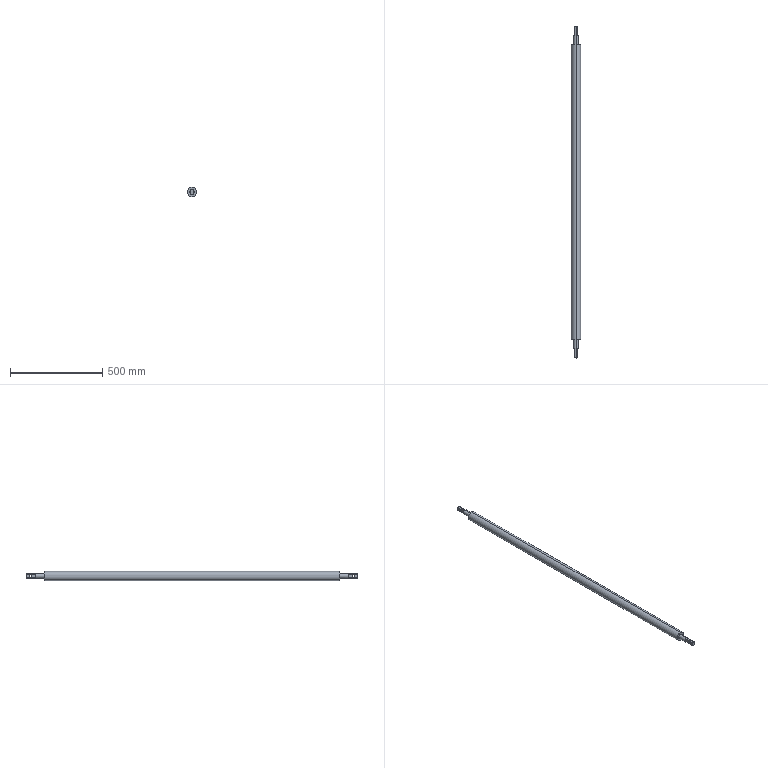Part | STEP file | Roller 11 | 1 solid | 22 faces | box 50 x 1800 x 50 mm | volume 3218952 mm3 | plane 12 | cylinder 10 | commonest cylinder face diameters 13 x4 25 x4 50 x2
STEP:
#1=CARTESIAN_POINT('',(6.703,-875.,6.5));
#2=VERTEX_POINT('',#1);
#3=CARTESIAN_POINT('',(6.703,-875.,-6.5));
#4=VERTEX_POINT('',#3);
#5=CARTESIAN_POINT('',(6.703,-875.,0.));
#6=DIRECTION('',(1.,0.,0.));
#7=DIRECTION('',(0.,0.,1.));
#8=AXIS2_PLACEMENT_3D('',#5,#6,#7);
#9=CIRCLE('',#8,6.5);
#10=EDGE_CURVE('',#2,#4,#9,.T.);
#11=ORIENTED_EDGE('',*,*,#10,.T.);
#12=CARTESIAN_POINT('',(-6.703,-875.,-6.5));
#13=VERTEX_POINT('',#12);
#14=CARTESIAN_POINT('',(29.297,-875.,-6.5));
#15=DIRECTION('',(-1.,0.,0.));
#16=VECTOR('',#15,1000.);
#17=LINE('',#14,#16);
#18=EDGE_CURVE('',#4,#13,#17,.T.);
#19=ORIENTED_EDGE('',*,*,#18,.T.);
#20=CARTESIAN_POINT('',(-6.703,-875.,6.5));
#21=VERTEX_POINT('',#20);
#22=CARTESIAN_POINT('',(-6.703,-875.,0.));
#23=DIRECTION('',(1.,0.,0.));
#24=DIRECTION('',(0.,0.,1.));
#25=AXIS2_PLACEMENT_3D('',#22,#23,#24);
#26=CIRCLE('',#25,6.5);
#27=EDGE_CURVE('',#21,#13,#26,.T.);
#28=ORIENTED_EDGE('',*,*,#27,.F.);
#29=CARTESIAN_POINT('',(29.297,-875.,6.5));
#30=DIRECTION('',(-1.,0.,0.));
#31=VECTOR('',#30,1000.);
#32=LINE('',#29,#31);
#33=EDGE_CURVE('',#2,#21,#32,.T.);
#34=ORIENTED_EDGE('',*,*,#33,.F.);
#35=EDGE_LOOP('',(#11,#19,#28,#34));
#36=FACE_OUTER_BOUND('',#35,.T.);
#37=CARTESIAN_POINT('',(29.297,-875.,0.));
#38=DIRECTION('',(-1.,0.,0.));
#39=DIRECTION('',(0.,0.,1.));
#40=AXIS2_PLACEMENT_3D('',#37,#38,#39);
#41=CYLINDRICAL_SURFACE('',#40,6.5);
#42=ADVANCED_FACE('',(#36),#41,.F.);
#43=CARTESIAN_POINT('',(6.703,875.,6.5));
#44=VERTEX_POINT('',#43);
#45=CARTESIAN_POINT('',(6.703,875.,-6.5));
#46=VERTEX_POINT('',#45);
#47=CARTESIAN_POINT('',(6.703,875.,0.));
#48=DIRECTION('',(1.,0.,0.));
#49=DIRECTION('',(0.,0.,-1.));
#50=AXIS2_PLACEMENT_3D('',#47,#48,#49);
#51=CIRCLE('',#50,6.5);
#52=EDGE_CURVE('',#44,#46,#51,.T.);
#53=ORIENTED_EDGE('',*,*,#52,.T.);
#54=CARTESIAN_POINT('',(-6.703,875.,-6.5));
#55=VERTEX_POINT('',#54);
#56=CARTESIAN_POINT('',(29.297,875.,-6.5));
#57=DIRECTION('',(-1.,0.,0.));
#58=VECTOR('',#57,1000.);
#59=LINE('',#56,#58);
#60=EDGE_CURVE('',#46,#55,#59,.T.);
#61=ORIENTED_EDGE('',*,*,#60,.T.);
#62=CARTESIAN_POINT('',(-6.703,875.,6.5));
#63=VERTEX_POINT('',#62);
#64=CARTESIAN_POINT('',(-6.703,875.,0.));
#65=DIRECTION('',(-1.,0.,0.));
#66=DIRECTION('',(0.,0.,1.));
#67=AXIS2_PLACEMENT_3D('',#64,#65,#66);
#68=CIRCLE('',#67,6.5);
#69=EDGE_CURVE('',#55,#63,#68,.T.);
#70=ORIENTED_EDGE('',*,*,#69,.T.);
#71=CARTESIAN_POINT('',(29.297,875.,6.5));
#72=DIRECTION('',(-1.,0.,0.));
#73=VECTOR('',#72,1000.);
#74=LINE('',#71,#73);
#75=EDGE_CURVE('',#44,#63,#74,.T.);
#76=ORIENTED_EDGE('',*,*,#75,.F.);
#77=EDGE_LOOP('',(#53,#61,#70,#76));
#78=FACE_OUTER_BOUND('',#77,.T.);
#79=CARTESIAN_POINT('',(29.297,875.,0.));
#80=DIRECTION('',(-1.,0.,0.));
#81=DIRECTION('',(0.,0.,1.));
#82=AXIS2_PLACEMENT_3D('',#79,#80,#81);
#83=CYLINDRICAL_SURFACE('',#82,6.5);
#84=ADVANCED_FACE('',(#78),#83,.F.);
#85=CARTESIAN_POINT('',(0.,-800.,-12.5));
#86=VERTEX_POINT('',#85);
#87=CARTESIAN_POINT('',(0.,-800.,12.5));
#88=VERTEX_POINT('',#87);
#89=CARTESIAN_POINT('',(0.,-800.,0.));
#90=DIRECTION('',(0.,-1.,0.));
#91=DIRECTION('',(0.,0.,1.));
#92=AXIS2_PLACEMENT_3D('',#89,#90,#91);
#93=CIRCLE('',#92,12.5);
#94=EDGE_CURVE('',#86,#88,#93,.T.);
#95=ORIENTED_EDGE('',*,*,#94,.T.);
#96=CARTESIAN_POINT('',(0.,-900.,12.5));
#97=VERTEX_POINT('',#96);
#98=CARTESIAN_POINT('',(0.,900.,12.5));
#99=DIRECTION('',(0.,-1.,0.));
#100=VECTOR('',#99,1000.);
#101=LINE('',#98,#100);
#102=EDGE_CURVE('',#88,#97,#101,.T.);
#103=ORIENTED_EDGE('',*,*,#102,.T.);
#104=CARTESIAN_POINT('',(6.703,-900.,10.551));
#105=VERTEX_POINT('',#104);
#106=CARTESIAN_POINT('',(0.,-900.,0.));
#107=DIRECTION('',(0.,1.,0.));
#108=DIRECTION('',(0.,0.,1.));
#109=AXIS2_PLACEMENT_3D('',#106,#107,#108);
#110=CIRCLE('',#109,12.5);
#111=EDGE_CURVE('',#97,#105,#110,.T.);
#112=ORIENTED_EDGE('',*,*,#111,.T.);
#113=CARTESIAN_POINT('',(6.703,-850.,10.551));
#114=VERTEX_POINT('',#113);
#115=CARTESIAN_POINT('',(6.703,900.,10.551));
#116=DIRECTION('',(0.,1.,0.));
#117=VECTOR('',#116,1000.);
#118=LINE('',#115,#117);
#119=EDGE_CURVE('',#105,#114,#118,.T.);
#120=ORIENTED_EDGE('',*,*,#119,.T.);
#121=CARTESIAN_POINT('',(6.703,-850.,-10.551));
#122=VERTEX_POINT('',#121);
#123=CARTESIAN_POINT('',(0.,-850.,0.));
#124=DIRECTION('',(0.,-1.,0.));
#125=DIRECTION('',(0.,0.,-1.));
#126=AXIS2_PLACEMENT_3D('',#123,#124,#125);
#127=CIRCLE('',#126,12.5);
#128=EDGE_CURVE('',#122,#114,#127,.T.);
#129=ORIENTED_EDGE('',*,*,#128,.F.);
#130=CARTESIAN_POINT('',(6.703,-900.,-10.551));
#131=VERTEX_POINT('',#130);
#132=CARTESIAN_POINT('',(6.703,900.,-10.551));
#133=DIRECTION('',(0.,-1.,0.));
#134=VECTOR('',#133,1000.);
#135=LINE('',#132,#134);
#136=EDGE_CURVE('',#122,#131,#135,.T.);
#137=ORIENTED_EDGE('',*,*,#136,.T.);
#138=CARTESIAN_POINT('',(0.,-900.,-12.5));
#139=VERTEX_POINT('',#138);
#140=CARTESIAN_POINT('',(0.,-900.,0.));
#141=DIRECTION('',(0.,1.,0.));
#142=DIRECTION('',(0.,0.,1.));
#143=AXIS2_PLACEMENT_3D('',#140,#141,#142);
#144=CIRCLE('',#143,12.5);
#145=EDGE_CURVE('',#131,#139,#144,.T.);
#146=ORIENTED_EDGE('',*,*,#145,.T.);
#147=CARTESIAN_POINT('',(0.,900.,-12.5));
#148=DIRECTION('',(0.,-1.,0.));
#149=VECTOR('',#148,1000.);
#150=LINE('',#147,#149);
#151=EDGE_CURVE('',#86,#139,#150,.T.);
#152=ORIENTED_EDGE('',*,*,#151,.F.);
#153=EDGE_LOOP('',(#95,#103,#112,#120,#129,#137,#146,#152));
#154=FACE_OUTER_BOUND('',#153,.T.);
#155=CARTESIAN_POINT('',(0.,900.,0.));
#156=DIRECTION('',(0.,-1.,0.));
#157=DIRECTION('',(0.,0.,-1.));
#158=AXIS2_PLACEMENT_3D('',#155,#156,#157);
#159=CYLINDRICAL_SURFACE('',#158,12.5);
#160=ADVANCED_FACE('',(#154),#159,.T.);
#161=CARTESIAN_POINT('',(0.,800.,25.));
#162=VERTEX_POINT('',#161);
#163=CARTESIAN_POINT('',(0.,800.,-25.));
#164=VERTEX_POINT('',#163);
#165=CARTESIAN_POINT('',(0.,800.,0.));
#166=DIRECTION('',(0.,1.,0.));
#167=DIRECTION('',(0.,0.,1.));
#168=AXIS2_PLACEMENT_3D('',#165,#166,#167);
#169=CIRCLE('',#168,25.);
#170=EDGE_CURVE('',#162,#164,#169,.T.);
#171=ORIENTED_EDGE('',*,*,#170,.F.);
#172=CARTESIAN_POINT('',(0.,-800.,25.));
#173=VERTEX_POINT('',#172);
#174=CARTESIAN_POINT('',(0.,800.,25.));
#175=DIRECTION('',(0.,-1.,0.));
#176=VECTOR('',#175,1000.);
#177=LINE('',#174,#176);
#178=EDGE_CURVE('',#162,#173,#177,.T.);
#179=ORIENTED_EDGE('',*,*,#178,.T.);
#180=CARTESIAN_POINT('',(0.,-800.,-25.));
#181=VERTEX_POINT('',#180);
#182=CARTESIAN_POINT('',(0.,-800.,0.));
#183=DIRECTION('',(0.,1.,0.));
#184=DIRECTION('',(0.,0.,1.));
#185=AXIS2_PLACEMENT_3D('',#182,#183,#184);
#186=CIRCLE('',#185,25.);
#187=EDGE_CURVE('',#173,#181,#186,.T.);
#188=ORIENTED_EDGE('',*,*,#187,.T.);
#189=CARTESIAN_POINT('',(0.,800.,-25.));
#190=DIRECTION('',(0.,-1.,0.));
#191=VECTOR('',#190,1000.);
#192=LINE('',#189,#191);
#193=EDGE_CURVE('',#164,#181,#192,.T.);
#194=ORIENTED_EDGE('',*,*,#193,.F.);
#195=EDGE_LOOP('',(#171,#179,#188,#194));
#196=FACE_OUTER_BOUND('',#195,.T.);
#197=CARTESIAN_POINT('',(0.,800.,0.));
#198=DIRECTION('',(0.,-1.,0.));
#199=DIRECTION('',(0.,0.,-1.));
#200=AXIS2_PLACEMENT_3D('',#197,#198,#199);
#201=CYLINDRICAL_SURFACE('',#200,25.);
#202=ADVANCED_FACE('',(#196),#201,.T.);
#203=CARTESIAN_POINT('',(0.,900.,12.5));
#204=VERTEX_POINT('',#203);
#205=CARTESIAN_POINT('',(6.703,900.,10.551));
#206=VERTEX_POINT('',#205);
#207=CARTESIAN_POINT('',(0.,900.,0.));
#208=DIRECTION('',(0.,1.,0.));
#209=DIRECTION('',(0.,0.,1.));
#210=AXIS2_PLACEMENT_3D('',#207,#208,#209);
#211=CIRCLE('',#210,12.5);
#212=EDGE_CURVE('',#204,#206,#211,.T.);
#213=ORIENTED_EDGE('',*,*,#212,.F.);
#214=CARTESIAN_POINT('',(0.,800.,12.5));
#215=VERTEX_POINT('',#214);
#216=CARTESIAN_POINT('',(0.,900.,12.5));
#217=DIRECTION('',(0.,-1.,0.));
#218=VECTOR('',#217,1000.);
#219=LINE('',#216,#218);
#220=EDGE_CURVE('',#204,#215,#219,.T.);
#221=ORIENTED_EDGE('',*,*,#220,.T.);
#222=CARTESIAN_POINT('',(0.,800.,-12.5));
#223=VERTEX_POINT('',#222);
#224=CARTESIAN_POINT('',(0.,800.,0.));
#225=DIRECTION('',(0.,-1.,0.));
#226=DIRECTION('',(0.,0.,1.));
#227=AXIS2_PLACEMENT_3D('',#224,#225,#226);
#228=CIRCLE('',#227,12.5);
#229=EDGE_CURVE('',#223,#215,#228,.T.);
#230=ORIENTED_EDGE('',*,*,#229,.F.);
#231=CARTESIAN_POINT('',(0.,900.,-12.5));
#232=VERTEX_POINT('',#231);
#233=CARTESIAN_POINT('',(0.,900.,-12.5));
#234=DIRECTION('',(0.,-1.,0.));
#235=VECTOR('',#234,1000.);
#236=LINE('',#233,#235);
#237=EDGE_CURVE('',#232,#223,#236,.T.);
#238=ORIENTED_EDGE('',*,*,#237,.F.);
#239=CARTESIAN_POINT('',(6.703,900.,-10.551));
#240=VERTEX_POINT('',#239);
#241=CARTESIAN_POINT('',(0.,900.,0.));
#242=DIRECTION('',(0.,1.,0.));
#243=DIRECTION('',(0.,0.,1.));
#244=AXIS2_PLACEMENT_3D('',#241,#242,#243);
#245=CIRCLE('',#244,12.5);
#246=EDGE_CURVE('',#240,#232,#245,.T.);
#247=ORIENTED_EDGE('',*,*,#246,.F.);
#248=CARTESIAN_POINT('',(6.703,850.,-10.551));
#249=VERTEX_POINT('',#248);
#250=CARTESIAN_POINT('',(6.703,900.,-10.551));
#251=DIRECTION('',(0.,1.,0.));
#252=VECTOR('',#251,1000.);
#253=LINE('',#250,#252);
#254=EDGE_CURVE('',#249,#240,#253,.T.);
#255=ORIENTED_EDGE('',*,*,#254,.F.);
#256=CARTESIAN_POINT('',(6.703,850.,10.551));
#257=VERTEX_POINT('',#256);
#258=CARTESIAN_POINT('',(0.,850.,0.));
#259=DIRECTION('',(0.,1.,0.));
#260=DIRECTION('',(0.,0.,1.));
#261=AXIS2_PLACEMENT_3D('',#258,#259,#260);
#262=CIRCLE('',#261,12.5);
#263=EDGE_CURVE('',#257,#249,#262,.T.);
#264=ORIENTED_EDGE('',*,*,#263,.F.);
#265=CARTESIAN_POINT('',(6.703,900.,10.551));
#266=DIRECTION('',(0.,-1.,0.));
#267=VECTOR('',#266,1000.);
#268=LINE('',#265,#267);
#269=EDGE_CURVE('',#206,#257,#268,.T.);
#270=ORIENTED_EDGE('',*,*,#269,.F.);
#271=EDGE_LOOP('',(#213,#221,#230,#238,#247,#255,#264,#270));
#272=FACE_OUTER_BOUND('',#271,.T.);
#273=CARTESIAN_POINT('',(0.,900.,0.));
#274=DIRECTION('',(0.,-1.,0.));
#275=DIRECTION('',(0.,0.,-1.));
#276=AXIS2_PLACEMENT_3D('',#273,#274,#275);
#277=CYLINDRICAL_SURFACE('',#276,12.5);
#278=ADVANCED_FACE('',(#272),#277,.T.);
#279=ORIENTED_EDGE('',*,*,#220,.F.);
#280=CARTESIAN_POINT('',(-6.703,900.,10.551));
#281=VERTEX_POINT('',#280);
#282=CARTESIAN_POINT('',(0.,900.,0.));
#283=DIRECTION('',(0.,1.,0.));
#284=DIRECTION('',(0.,0.,1.));
#285=AXIS2_PLACEMENT_3D('',#282,#283,#284);
#286=CIRCLE('',#285,12.5);
#287=EDGE_CURVE('',#281,#204,#286,.T.);
#288=ORIENTED_EDGE('',*,*,#287,.F.);
#289=CARTESIAN_POINT('',(-6.703,850.,10.551));
#290=VERTEX_POINT('',#289);
#291=CARTESIAN_POINT('',(-6.703,900.,10.551));
#292=DIRECTION('',(0.,1.,0.));
#293=VECTOR('',#292,1000.);
#294=LINE('',#291,#293);
#295=EDGE_CURVE('',#290,#281,#294,.T.);
#296=ORIENTED_EDGE('',*,*,#295,.F.);
#297=CARTESIAN_POINT('',(-6.703,850.,-10.551));
#298=VERTEX_POINT('',#297);
#299=CARTESIAN_POINT('',(0.,850.,0.));
#300=DIRECTION('',(0.,1.,0.));
#301=DIRECTION('',(0.,0.,1.));
#302=AXIS2_PLACEMENT_3D('',#299,#300,#301);
#303=CIRCLE('',#302,12.5);
#304=EDGE_CURVE('',#298,#290,#303,.T.);
#305=ORIENTED_EDGE('',*,*,#304,.F.);
#306=CARTESIAN_POINT('',(-6.703,900.,-10.551));
#307=VERTEX_POINT('',#306);
#308=CARTESIAN_POINT('',(-6.703,900.,-10.551));
#309=DIRECTION('',(0.,-1.,0.));
#310=VECTOR('',#309,1000.);
#311=LINE('',#308,#310);
#312=EDGE_CURVE('',#307,#298,#311,.T.);
#313=ORIENTED_EDGE('',*,*,#312,.F.);
#314=CARTESIAN_POINT('',(0.,900.,0.));
#315=DIRECTION('',(0.,1.,0.));
#316=DIRECTION('',(0.,0.,1.));
#317=AXIS2_PLACEMENT_3D('',#314,#315,#316);
#318=CIRCLE('',#317,12.5);
#319=EDGE_CURVE('',#232,#307,#318,.T.);
#320=ORIENTED_EDGE('',*,*,#319,.F.);
#321=ORIENTED_EDGE('',*,*,#237,.T.);
#322=CARTESIAN_POINT('',(0.,800.,0.));
#323=DIRECTION('',(0.,-1.,0.));
#324=DIRECTION('',(0.,0.,1.));
#325=AXIS2_PLACEMENT_3D('',#322,#323,#324);
#326=CIRCLE('',#325,12.5);
#327=EDGE_CURVE('',#215,#223,#326,.T.);
#328=ORIENTED_EDGE('',*,*,#327,.F.);
#329=EDGE_LOOP('',(#279,#288,#296,#305,#313,#320,#321,#328));
#330=FACE_OUTER_BOUND('',#329,.T.);
#331=CARTESIAN_POINT('',(0.,900.,0.));
#332=DIRECTION('',(0.,-1.,0.));
#333=DIRECTION('',(0.,0.,-1.));
#334=AXIS2_PLACEMENT_3D('',#331,#332,#333);
#335=CYLINDRICAL_SURFACE('',#334,12.5);
#336=ADVANCED_FACE('',(#330),#335,.T.);
#337=ORIENTED_EDGE('',*,*,#246,.T.);
#338=ORIENTED_EDGE('',*,*,#319,.T.);
#339=CARTESIAN_POINT('',(-6.703,900.,0.));
#340=DIRECTION('',(0.,0.,1.));
#341=VECTOR('',#340,1000.);
#342=LINE('',#339,#341);
#343=EDGE_CURVE('',#307,#281,#342,.T.);
#344=ORIENTED_EDGE('',*,*,#343,.T.);
#345=ORIENTED_EDGE('',*,*,#287,.T.);
#346=ORIENTED_EDGE('',*,*,#212,.T.);
#347=CARTESIAN_POINT('',(6.703,900.,0.));
#348=DIRECTION('',(0.,0.,-1.));
#349=VECTOR('',#348,1000.);
#350=LINE('',#347,#349);
#351=EDGE_CURVE('',#206,#240,#350,.T.);
#352=ORIENTED_EDGE('',*,*,#351,.T.);
#353=EDGE_LOOP('',(#337,#338,#344,#345,#346,#352));
#354=FACE_OUTER_BOUND('',#353,.T.);
#355=CARTESIAN_POINT('',(0.,900.,0.));
#356=DIRECTION('',(0.,1.,0.));
#357=DIRECTION('',(0.,0.,1.));
#358=AXIS2_PLACEMENT_3D('',#355,#356,#357);
#359=PLANE('',#358);
#360=ADVANCED_FACE('',(#354),#359,.T.);
#361=ORIENTED_EDGE('',*,*,#178,.F.);
#362=CARTESIAN_POINT('',(0.,800.,0.));
#363=DIRECTION('',(0.,1.,0.));
#364=DIRECTION('',(0.,0.,1.));
#365=AXIS2_PLACEMENT_3D('',#362,#363,#364);
#366=CIRCLE('',#365,25.);
#367=EDGE_CURVE('',#164,#162,#366,.T.);
#368=ORIENTED_EDGE('',*,*,#367,.F.);
#369=ORIENTED_EDGE('',*,*,#193,.T.);
#370=CARTESIAN_POINT('',(0.,-800.,0.));
#371=DIRECTION('',(0.,1.,0.));
#372=DIRECTION('',(0.,0.,1.));
#373=AXIS2_PLACEMENT_3D('',#370,#371,#372);
#374=CIRCLE('',#373,25.);
#375=EDGE_CURVE('',#181,#173,#374,.T.);
#376=ORIENTED_EDGE('',*,*,#375,.T.);
#377=EDGE_LOOP('',(#361,#368,#369,#376));
#378=FACE_OUTER_BOUND('',#377,.T.);
#379=CARTESIAN_POINT('',(0.,800.,0.));
#380=DIRECTION('',(0.,-1.,0.));
#381=DIRECTION('',(0.,0.,-1.));
#382=AXIS2_PLACEMENT_3D('',#379,#380,#381);
#383=CYLINDRICAL_SURFACE('',#382,25.);
#384=ADVANCED_FACE('',(#378),#383,.T.);
#385=ORIENTED_EDGE('',*,*,#229,.T.);
#386=ORIENTED_EDGE('',*,*,#327,.T.);
#387=EDGE_LOOP('',(#385,#386));
#388=FACE_BOUND('',#387,.T.);
#389=ORIENTED_EDGE('',*,*,#367,.T.);
#390=ORIENTED_EDGE('',*,*,#170,.T.);
#391=EDGE_LOOP('',(#389,#390));
#392=FACE_OUTER_BOUND('',#391,.T.);
#393=CARTESIAN_POINT('',(0.,800.,0.));
#394=DIRECTION('',(0.,1.,0.));
#395=DIRECTION('',(0.,0.,1.));
#396=AXIS2_PLACEMENT_3D('',#393,#394,#395);
#397=PLANE('',#396);
#398=ADVANCED_FACE('',(#388,#392),#397,.T.);
#399=ORIENTED_EDGE('',*,*,#94,.F.);
#400=CARTESIAN_POINT('',(0.,-800.,0.));
#401=DIRECTION('',(0.,-1.,0.));
#402=DIRECTION('',(0.,0.,1.));
#403=AXIS2_PLACEMENT_3D('',#400,#401,#402);
#404=CIRCLE('',#403,12.5);
#405=EDGE_CURVE('',#88,#86,#404,.T.);
#406=ORIENTED_EDGE('',*,*,#405,.F.);
#407=EDGE_LOOP('',(#399,#406));
#408=FACE_BOUND('',#407,.T.);
#409=ORIENTED_EDGE('',*,*,#375,.F.);
#410=ORIENTED_EDGE('',*,*,#187,.F.);
#411=EDGE_LOOP('',(#409,#410));
#412=FACE_OUTER_BOUND('',#411,.T.);
#413=CARTESIAN_POINT('',(0.,-800.,0.));
#414=DIRECTION('',(0.,1.,0.));
#415=DIRECTION('',(0.,0.,1.));
#416=AXIS2_PLACEMENT_3D('',#413,#414,#415);
#417=PLANE('',#416);
#418=ADVANCED_FACE('',(#408,#412),#417,.F.);
#419=CARTESIAN_POINT('',(-6.703,-900.,10.551));
#420=VERTEX_POINT('',#419);
#421=CARTESIAN_POINT('',(0.,-900.,0.));
#422=DIRECTION('',(0.,1.,0.));
#423=DIRECTION('',(0.,0.,1.));
#424=AXIS2_PLACEMENT_3D('',#421,#422,#423);
#425=CIRCLE('',#424,12.5);
#426=EDGE_CURVE('',#420,#97,#425,.T.);
#427=ORIENTED_EDGE('',*,*,#426,.F.);
#428=CARTESIAN_POINT('',(-6.703,-900.,-10.551));
#429=VERTEX_POINT('',#428);
#430=CARTESIAN_POINT('',(-6.703,-900.,-19.04));
#431=DIRECTION('',(0.,0.,1.));
#432=VECTOR('',#431,1000.);
#433=LINE('',#430,#432);
#434=EDGE_CURVE('',#429,#420,#433,.T.);
#435=ORIENTED_EDGE('',*,*,#434,.F.);
#436=CARTESIAN_POINT('',(0.,-900.,0.));
#437=DIRECTION('',(0.,1.,0.));
#438=DIRECTION('',(0.,0.,1.));
#439=AXIS2_PLACEMENT_3D('',#436,#437,#438);
#440=CIRCLE('',#439,12.5);
#441=EDGE_CURVE('',#139,#429,#440,.T.);
#442=ORIENTED_EDGE('',*,*,#441,.F.);
#443=ORIENTED_EDGE('',*,*,#145,.F.);
#444=CARTESIAN_POINT('',(6.703,-900.,-19.04));
#445=DIRECTION('',(0.,0.,-1.));
#446=VECTOR('',#445,1000.);
#447=LINE('',#444,#446);
#448=EDGE_CURVE('',#105,#131,#447,.T.);
#449=ORIENTED_EDGE('',*,*,#448,.F.);
#450=ORIENTED_EDGE('',*,*,#111,.F.);
#451=EDGE_LOOP('',(#427,#435,#442,#443,#449,#450));
#452=FACE_OUTER_BOUND('',#451,.T.);
#453=CARTESIAN_POINT('',(0.,-900.,0.));
#454=DIRECTION('',(0.,1.,0.));
#455=DIRECTION('',(0.,0.,1.));
#456=AXIS2_PLACEMENT_3D('',#453,#454,#455);
#457=PLANE('',#456);
#458=ADVANCED_FACE('',(#452),#457,.F.);
#459=ORIENTED_EDGE('',*,*,#102,.F.);
#460=ORIENTED_EDGE('',*,*,#405,.T.);
#461=ORIENTED_EDGE('',*,*,#151,.T.);
#462=ORIENTED_EDGE('',*,*,#441,.T.);
#463=CARTESIAN_POINT('',(-6.703,-850.,-10.551));
#464=VERTEX_POINT('',#463);
#465=CARTESIAN_POINT('',(-6.703,900.,-10.551));
#466=DIRECTION('',(0.,1.,0.));
#467=VECTOR('',#466,1000.);
#468=LINE('',#465,#467);
#469=EDGE_CURVE('',#429,#464,#468,.T.);
#470=ORIENTED_EDGE('',*,*,#469,.T.);
#471=CARTESIAN_POINT('',(-6.703,-850.,10.551));
#472=VERTEX_POINT('',#471);
#473=CARTESIAN_POINT('',(0.,-850.,0.));
#474=DIRECTION('',(0.,-1.,0.));
#475=DIRECTION('',(0.,0.,-1.));
#476=AXIS2_PLACEMENT_3D('',#473,#474,#475);
#477=CIRCLE('',#476,12.5);
#478=EDGE_CURVE('',#472,#464,#477,.T.);
#479=ORIENTED_EDGE('',*,*,#478,.F.);
#480=CARTESIAN_POINT('',(-6.703,900.,10.551));
#481=DIRECTION('',(0.,-1.,0.));
#482=VECTOR('',#481,1000.);
#483=LINE('',#480,#482);
#484=EDGE_CURVE('',#472,#420,#483,.T.);
#485=ORIENTED_EDGE('',*,*,#484,.T.);
#486=ORIENTED_EDGE('',*,*,#426,.T.);
#487=EDGE_LOOP('',(#459,#460,#461,#462,#470,#479,#485,#486));
#488=FACE_OUTER_BOUND('',#487,.T.);
#489=CARTESIAN_POINT('',(0.,900.,0.));
#490=DIRECTION('',(0.,-1.,0.));
#491=DIRECTION('',(0.,0.,-1.));
#492=AXIS2_PLACEMENT_3D('',#489,#490,#491);
#493=CYLINDRICAL_SURFACE('',#492,12.5);
#494=ADVANCED_FACE('',(#488),#493,.T.);
#495=ORIENTED_EDGE('',*,*,#52,.F.);
#496=CARTESIAN_POINT('',(6.703,875.,0.));
#497=DIRECTION('',(1.,0.,0.));
#498=DIRECTION('',(0.,0.,-1.));
#499=AXIS2_PLACEMENT_3D('',#496,#497,#498);
#500=CIRCLE('',#499,6.5);
#501=EDGE_CURVE('',#46,#44,#500,.T.);
#502=ORIENTED_EDGE('',*,*,#501,.F.);
#503=EDGE_LOOP('',(#495,#502));
#504=FACE_BOUND('',#503,.T.);
#505=ORIENTED_EDGE('',*,*,#269,.T.);
#506=CARTESIAN_POINT('',(6.703,850.,-19.04));
#507=DIRECTION('',(0.,0.,-1.));
#508=VECTOR('',#507,1000.);
#509=LINE('',#506,#508);
#510=EDGE_CURVE('',#257,#249,#509,.T.);
#511=ORIENTED_EDGE('',*,*,#510,.T.);
#512=ORIENTED_EDGE('',*,*,#254,.T.);
#513=ORIENTED_EDGE('',*,*,#351,.F.);
#514=EDGE_LOOP('',(#505,#511,#512,#513));
#515=FACE_OUTER_BOUND('',#514,.T.);
#516=CARTESIAN_POINT('',(6.703,850.,-19.04));
#517=DIRECTION('',(1.,0.,0.));
#518=DIRECTION('',(0.,0.,-1.));
#519=AXIS2_PLACEMENT_3D('',#516,#517,#518);
#520=PLANE('',#519);
#521=ADVANCED_FACE('',(#504,#515),#520,.T.);
#522=ORIENTED_EDGE('',*,*,#263,.T.);
#523=ORIENTED_EDGE('',*,*,#510,.F.);
#524=EDGE_LOOP('',(#522,#523));
#525=FACE_OUTER_BOUND('',#524,.T.);
#526=CARTESIAN_POINT('',(0.,850.,0.));
#527=DIRECTION('',(0.,1.,0.));
#528=DIRECTION('',(0.,0.,1.));
#529=AXIS2_PLACEMENT_3D('',#526,#527,#528);
#530=PLANE('',#529);
#531=ADVANCED_FACE('',(#525),#530,.T.);
#532=ORIENTED_EDGE('',*,*,#304,.T.);
#533=CARTESIAN_POINT('',(-6.703,850.,-19.04));
#534=DIRECTION('',(0.,0.,1.));
#535=VECTOR('',#534,1000.);
#536=LINE('',#533,#535);
#537=EDGE_CURVE('',#298,#290,#536,.T.);
#538=ORIENTED_EDGE('',*,*,#537,.F.);
#539=EDGE_LOOP('',(#532,#538));
#540=FACE_OUTER_BOUND('',#539,.T.);
#541=CARTESIAN_POINT('',(0.,850.,0.));
#542=DIRECTION('',(0.,1.,0.));
#543=DIRECTION('',(0.,0.,1.));
#544=AXIS2_PLACEMENT_3D('',#541,#542,#543);
#545=PLANE('',#544);
#546=ADVANCED_FACE('',(#540),#545,.T.);
#547=CARTESIAN_POINT('',(-6.703,875.,0.));
#548=DIRECTION('',(-1.,0.,0.));
#549=DIRECTION('',(0.,0.,1.));
#550=AXIS2_PLACEMENT_3D('',#547,#548,#549);
#551=CIRCLE('',#550,6.5);
#552=EDGE_CURVE('',#63,#55,#551,.T.);
#553=ORIENTED_EDGE('',*,*,#552,.F.);
#554=ORIENTED_EDGE('',*,*,#69,.F.);
#555=EDGE_LOOP('',(#553,#554));
#556=FACE_BOUND('',#555,.T.);
#557=ORIENTED_EDGE('',*,*,#312,.T.);
#558=ORIENTED_EDGE('',*,*,#537,.T.);
#559=ORIENTED_EDGE('',*,*,#295,.T.);
#560=ORIENTED_EDGE('',*,*,#343,.F.);
#561=EDGE_LOOP('',(#557,#558,#559,#560));
#562=FACE_OUTER_BOUND('',#561,.T.);
#563=CARTESIAN_POINT('',(-6.703,850.,-19.04));
#564=DIRECTION('',(-1.,0.,0.));
#565=DIRECTION('',(0.,0.,1.));
#566=AXIS2_PLACEMENT_3D('',#563,#564,#565);
#567=PLANE('',#566);
#568=ADVANCED_FACE('',(#556,#562),#567,.T.);
#569=ORIENTED_EDGE('',*,*,#60,.F.);
#570=ORIENTED_EDGE('',*,*,#501,.T.);
#571=ORIENTED_EDGE('',*,*,#75,.T.);
#572=ORIENTED_EDGE('',*,*,#552,.T.);
#573=EDGE_LOOP('',(#569,#570,#571,#572));
#574=FACE_OUTER_BOUND('',#573,.T.);
#575=CARTESIAN_POINT('',(29.297,875.,0.));
#576=DIRECTION('',(-1.,0.,0.));
#577=DIRECTION('',(0.,0.,1.));
#578=AXIS2_PLACEMENT_3D('',#575,#576,#577);
#579=CYLINDRICAL_SURFACE('',#578,6.5);
#580=ADVANCED_FACE('',(#574),#579,.F.);
#581=ORIENTED_EDGE('',*,*,#10,.F.);
#582=CARTESIAN_POINT('',(6.703,-875.,0.));
#583=DIRECTION('',(1.,0.,0.));
#584=DIRECTION('',(0.,0.,1.));
#585=AXIS2_PLACEMENT_3D('',#582,#583,#584);
#586=CIRCLE('',#585,6.5);
#587=EDGE_CURVE('',#4,#2,#586,.T.);
#588=ORIENTED_EDGE('',*,*,#587,.F.);
#589=EDGE_LOOP('',(#581,#588));
#590=FACE_BOUND('',#589,.T.);
#591=CARTESIAN_POINT('',(6.703,-850.,-19.04));
#592=DIRECTION('',(0.,0.,-1.));
#593=VECTOR('',#592,1000.);
#594=LINE('',#591,#593);
#595=EDGE_CURVE('',#114,#122,#594,.T.);
#596=ORIENTED_EDGE('',*,*,#595,.F.);
#597=ORIENTED_EDGE('',*,*,#119,.F.);
#598=ORIENTED_EDGE('',*,*,#448,.T.);
#599=ORIENTED_EDGE('',*,*,#136,.F.);
#600=EDGE_LOOP('',(#596,#597,#598,#599));
#601=FACE_OUTER_BOUND('',#600,.T.);
#602=CARTESIAN_POINT('',(6.703,-850.,-19.04));
#603=DIRECTION('',(-1.,0.,0.));
#604=DIRECTION('',(0.,0.,1.));
#605=AXIS2_PLACEMENT_3D('',#602,#603,#604);
#606=PLANE('',#605);
#607=ADVANCED_FACE('',(#590,#601),#606,.F.);
#608=ORIENTED_EDGE('',*,*,#128,.T.);
#609=ORIENTED_EDGE('',*,*,#595,.T.);
#610=EDGE_LOOP('',(#608,#609));
#611=FACE_OUTER_BOUND('',#610,.T.);
#612=CARTESIAN_POINT('',(0.,-850.,0.));
#613=DIRECTION('',(0.,-1.,0.));
#614=DIRECTION('',(0.,0.,-1.));
#615=AXIS2_PLACEMENT_3D('',#612,#613,#614);
#616=PLANE('',#615);
#617=ADVANCED_FACE('',(#611),#616,.T.);
#618=ORIENTED_EDGE('',*,*,#478,.T.);
#619=CARTESIAN_POINT('',(-6.703,-850.,-19.04));
#620=DIRECTION('',(0.,0.,1.));
#621=VECTOR('',#620,1000.);
#622=LINE('',#619,#621);
#623=EDGE_CURVE('',#464,#472,#622,.T.);
#624=ORIENTED_EDGE('',*,*,#623,.T.);
#625=EDGE_LOOP('',(#618,#624));
#626=FACE_OUTER_BOUND('',#625,.T.);
#627=CARTESIAN_POINT('',(0.,-850.,0.));
#628=DIRECTION('',(0.,-1.,0.));
#629=DIRECTION('',(0.,0.,-1.));
#630=AXIS2_PLACEMENT_3D('',#627,#628,#629);
#631=PLANE('',#630);
#632=ADVANCED_FACE('',(#626),#631,.T.);
#633=ORIENTED_EDGE('',*,*,#27,.T.);
#634=CARTESIAN_POINT('',(-6.703,-875.,0.));
#635=DIRECTION('',(1.,0.,0.));
#636=DIRECTION('',(0.,0.,1.));
#637=AXIS2_PLACEMENT_3D('',#634,#635,#636);
#638=CIRCLE('',#637,6.5);
#639=EDGE_CURVE('',#13,#21,#638,.T.);
#640=ORIENTED_EDGE('',*,*,#639,.T.);
#641=EDGE_LOOP('',(#633,#640));
#642=FACE_BOUND('',#641,.T.);
#643=ORIENTED_EDGE('',*,*,#623,.F.);
#644=ORIENTED_EDGE('',*,*,#469,.F.);
#645=ORIENTED_EDGE('',*,*,#434,.T.);
#646=ORIENTED_EDGE('',*,*,#484,.F.);
#647=EDGE_LOOP('',(#643,#644,#645,#646));
#648=FACE_OUTER_BOUND('',#647,.T.);
#649=CARTESIAN_POINT('',(-6.703,-850.,-19.04));
#650=DIRECTION('',(1.,0.,0.));
#651=DIRECTION('',(0.,0.,-1.));
#652=AXIS2_PLACEMENT_3D('',#649,#650,#651);
#653=PLANE('',#652);
#654=ADVANCED_FACE('',(#642,#648),#653,.F.);
#655=ORIENTED_EDGE('',*,*,#18,.F.);
#656=ORIENTED_EDGE('',*,*,#587,.T.);
#657=ORIENTED_EDGE('',*,*,#33,.T.);
#658=ORIENTED_EDGE('',*,*,#639,.F.);
#659=EDGE_LOOP('',(#655,#656,#657,#658));
#660=FACE_OUTER_BOUND('',#659,.T.);
#661=CARTESIAN_POINT('',(29.297,-875.,0.));
#662=DIRECTION('',(-1.,0.,0.));
#663=DIRECTION('',(0.,0.,1.));
#664=AXIS2_PLACEMENT_3D('',#661,#662,#663);
#665=CYLINDRICAL_SURFACE('',#664,6.5);
#666=ADVANCED_FACE('',(#660),#665,.F.);
#667=CLOSED_SHELL('',(#42,#84,#160,#202,#278,#336,#360,#384,#398,#418,#458,#494,#521,#531,#546,#568,#580,#607,#617,#632,#654,#666));
#668=MANIFOLD_SOLID_BREP('',#667);
#669=CARTESIAN_POINT('',(0.,0.,0.));
#670=DIRECTION('',(0.,0.,1.));
#671=DIRECTION('',(1.,0.,0.));
#672=AXIS2_PLACEMENT_3D('',#669,#670,#671);
#673=(LENGTH_UNIT()NAMED_UNIT(*)SI_UNIT(.MILLI.,.METRE.));
#674=UNCERTAINTY_MEASURE_WITH_UNIT(LENGTH_MEASURE(0.00001),#673,'','');
#675=(NAMED_UNIT(*)PLANE_ANGLE_UNIT()SI_UNIT($,.RADIAN.));
#676=(NAMED_UNIT(*)SI_UNIT($,.STERADIAN.)SOLID_ANGLE_UNIT());
#677=(GEOMETRIC_REPRESENTATION_CONTEXT(3)GLOBAL_UNCERTAINTY_ASSIGNED_CONTEXT((#674))GLOBAL_UNIT_ASSIGNED_CONTEXT((#673,#675,#676))REPRESENTATION_CONTEXT('',''));
#678=ADVANCED_BREP_SHAPE_REPRESENTATION('',(#668,#672),#677);